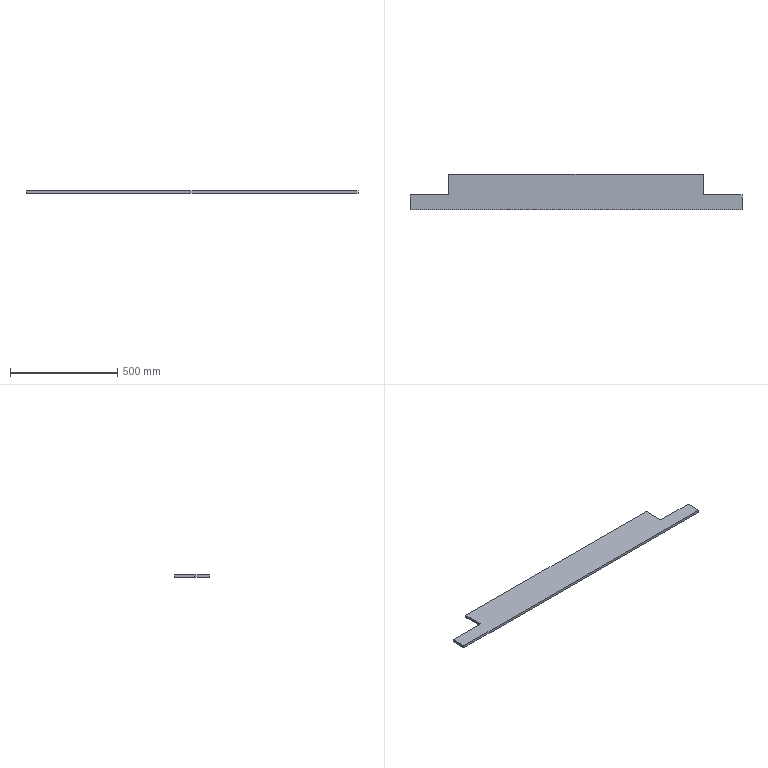Part | SolidWorks | features BaseBody 1 | 1 solid | 10 faces | box 1550 x 167 x 12 mm | volume 2687160 mm3 | plane 10
STEP:
#1=CARTESIAN_POINT('',(775.,-85.,-6.));
#2=VERTEX_POINT('',#1);
#3=CARTESIAN_POINT('',(775.,-15.,-6.));
#4=VERTEX_POINT('',#3);
#5=CARTESIAN_POINT('',(775.,85.,-6.));
#6=DIRECTION('',(0.,1.,0.));
#7=VECTOR('',#6,1000.);
#8=LINE('',#5,#7);
#9=EDGE_CURVE('',#2,#4,#8,.T.);
#10=ORIENTED_EDGE('',*,*,#9,.T.);
#11=CARTESIAN_POINT('',(775.,-15.,6.));
#12=VERTEX_POINT('',#11);
#13=CARTESIAN_POINT('',(775.,-15.,-8.));
#14=DIRECTION('',(0.,0.,1.));
#15=VECTOR('',#14,1000.);
#16=LINE('',#13,#15);
#17=EDGE_CURVE('',#4,#12,#16,.T.);
#18=ORIENTED_EDGE('',*,*,#17,.T.);
#19=CARTESIAN_POINT('',(775.,-85.,6.));
#20=VERTEX_POINT('',#19);
#21=CARTESIAN_POINT('',(775.,85.,6.));
#22=DIRECTION('',(0.,1.,0.));
#23=VECTOR('',#22,1000.);
#24=LINE('',#21,#23);
#25=EDGE_CURVE('',#20,#12,#24,.T.);
#26=ORIENTED_EDGE('',*,*,#25,.F.);
#27=CARTESIAN_POINT('',(775.,-85.,6.));
#28=DIRECTION('',(0.,0.,-1.));
#29=VECTOR('',#28,1000.);
#30=LINE('',#27,#29);
#31=EDGE_CURVE('',#20,#2,#30,.T.);
#32=ORIENTED_EDGE('',*,*,#31,.T.);
#33=EDGE_LOOP('',(#10,#18,#26,#32));
#34=FACE_OUTER_BOUND('',#33,.T.);
#35=CARTESIAN_POINT('',(775.,85.,6.));
#36=DIRECTION('',(-1.,0.,0.));
#37=DIRECTION('',(0.,0.,1.));
#38=AXIS2_PLACEMENT_3D('',#35,#36,#37);
#39=PLANE('',#38);
#40=ADVANCED_FACE('',(#34),#39,.F.);
#41=CARTESIAN_POINT('',(-775.,-15.,6.));
#42=VERTEX_POINT('',#41);
#43=CARTESIAN_POINT('',(-775.,-85.,6.));
#44=VERTEX_POINT('',#43);
#45=CARTESIAN_POINT('',(-775.,85.,6.));
#46=DIRECTION('',(0.,-1.,0.));
#47=VECTOR('',#46,1000.);
#48=LINE('',#45,#47);
#49=EDGE_CURVE('',#42,#44,#48,.T.);
#50=ORIENTED_EDGE('',*,*,#49,.F.);
#51=CARTESIAN_POINT('',(-775.,-15.,-6.));
#52=VERTEX_POINT('',#51);
#53=CARTESIAN_POINT('',(-775.,-15.,-8.));
#54=DIRECTION('',(0.,0.,1.));
#55=VECTOR('',#54,1000.);
#56=LINE('',#53,#55);
#57=EDGE_CURVE('',#52,#42,#56,.T.);
#58=ORIENTED_EDGE('',*,*,#57,.F.);
#59=CARTESIAN_POINT('',(-775.,-85.,-6.));
#60=VERTEX_POINT('',#59);
#61=CARTESIAN_POINT('',(-775.,85.,-6.));
#62=DIRECTION('',(0.,-1.,0.));
#63=VECTOR('',#62,1000.);
#64=LINE('',#61,#63);
#65=EDGE_CURVE('',#52,#60,#64,.T.);
#66=ORIENTED_EDGE('',*,*,#65,.T.);
#67=CARTESIAN_POINT('',(-775.,-85.,6.));
#68=DIRECTION('',(0.,0.,-1.));
#69=VECTOR('',#68,1000.);
#70=LINE('',#67,#69);
#71=EDGE_CURVE('',#44,#60,#70,.T.);
#72=ORIENTED_EDGE('',*,*,#71,.F.);
#73=EDGE_LOOP('',(#50,#58,#66,#72));
#74=FACE_OUTER_BOUND('',#73,.T.);
#75=CARTESIAN_POINT('',(-775.,85.,6.));
#76=DIRECTION('',(1.,0.,0.));
#77=DIRECTION('',(0.,0.,-1.));
#78=AXIS2_PLACEMENT_3D('',#75,#76,#77);
#79=PLANE('',#78);
#80=ADVANCED_FACE('',(#74),#79,.F.);
#81=CARTESIAN_POINT('',(-775.,-85.,-6.));
#82=DIRECTION('',(1.,0.,0.));
#83=VECTOR('',#82,1000.);
#84=LINE('',#81,#83);
#85=EDGE_CURVE('',#60,#2,#84,.T.);
#86=ORIENTED_EDGE('',*,*,#85,.T.);
#87=ORIENTED_EDGE('',*,*,#31,.F.);
#88=CARTESIAN_POINT('',(-775.,-85.,6.));
#89=DIRECTION('',(1.,0.,0.));
#90=VECTOR('',#89,1000.);
#91=LINE('',#88,#90);
#92=EDGE_CURVE('',#44,#20,#91,.T.);
#93=ORIENTED_EDGE('',*,*,#92,.F.);
#94=ORIENTED_EDGE('',*,*,#71,.T.);
#95=EDGE_LOOP('',(#86,#87,#93,#94));
#96=FACE_OUTER_BOUND('',#95,.T.);
#97=CARTESIAN_POINT('',(-775.,-85.,6.));
#98=DIRECTION('',(0.,1.,0.));
#99=DIRECTION('',(0.,0.,1.));
#100=AXIS2_PLACEMENT_3D('',#97,#98,#99);
#101=PLANE('',#100);
#102=ADVANCED_FACE('',(#96),#101,.F.);
#103=CARTESIAN_POINT('',(-595.,82.,6.));
#104=VERTEX_POINT('',#103);
#105=CARTESIAN_POINT('',(595.,82.,6.));
#106=VERTEX_POINT('',#105);
#107=CARTESIAN_POINT('',(-595.,82.,6.));
#108=DIRECTION('',(1.,0.,0.));
#109=VECTOR('',#108,1000.);
#110=LINE('',#107,#109);
#111=EDGE_CURVE('',#104,#106,#110,.T.);
#112=ORIENTED_EDGE('',*,*,#111,.F.);
#113=CARTESIAN_POINT('',(-595.,-15.,6.));
#114=VERTEX_POINT('',#113);
#115=CARTESIAN_POINT('',(-595.,-15.,6.));
#116=DIRECTION('',(0.,1.,0.));
#117=VECTOR('',#116,1000.);
#118=LINE('',#115,#117);
#119=EDGE_CURVE('',#114,#104,#118,.T.);
#120=ORIENTED_EDGE('',*,*,#119,.F.);
#121=CARTESIAN_POINT('',(-775.,-15.,6.));
#122=DIRECTION('',(1.,0.,0.));
#123=VECTOR('',#122,1000.);
#124=LINE('',#121,#123);
#125=EDGE_CURVE('',#42,#114,#124,.T.);
#126=ORIENTED_EDGE('',*,*,#125,.F.);
#127=ORIENTED_EDGE('',*,*,#49,.T.);
#128=ORIENTED_EDGE('',*,*,#92,.T.);
#129=ORIENTED_EDGE('',*,*,#25,.T.);
#130=CARTESIAN_POINT('',(595.,-15.,6.));
#131=VERTEX_POINT('',#130);
#132=CARTESIAN_POINT('',(775.,-15.,6.));
#133=DIRECTION('',(1.,0.,0.));
#134=VECTOR('',#133,1000.);
#135=LINE('',#132,#134);
#136=EDGE_CURVE('',#131,#12,#135,.T.);
#137=ORIENTED_EDGE('',*,*,#136,.F.);
#138=CARTESIAN_POINT('',(595.,-15.,6.));
#139=DIRECTION('',(0.,-1.,0.));
#140=VECTOR('',#139,1000.);
#141=LINE('',#138,#140);
#142=EDGE_CURVE('',#106,#131,#141,.T.);
#143=ORIENTED_EDGE('',*,*,#142,.F.);
#144=EDGE_LOOP('',(#112,#120,#126,#127,#128,#129,#137,#143));
#145=FACE_OUTER_BOUND('',#144,.T.);
#146=CARTESIAN_POINT('',(0.,0.,6.));
#147=DIRECTION('',(0.,0.,1.));
#148=DIRECTION('',(1.,0.,0.));
#149=AXIS2_PLACEMENT_3D('',#146,#147,#148);
#150=PLANE('',#149);
#151=ADVANCED_FACE('',(#145),#150,.T.);
#152=CARTESIAN_POINT('',(-595.,-15.,-6.));
#153=VERTEX_POINT('',#152);
#154=CARTESIAN_POINT('',(-595.,82.,-6.));
#155=VERTEX_POINT('',#154);
#156=CARTESIAN_POINT('',(-595.,0.,-6.));
#157=DIRECTION('',(0.,1.,0.));
#158=VECTOR('',#157,1000.);
#159=LINE('',#156,#158);
#160=EDGE_CURVE('',#153,#155,#159,.T.);
#161=ORIENTED_EDGE('',*,*,#160,.T.);
#162=CARTESIAN_POINT('',(595.,82.,-6.));
#163=VERTEX_POINT('',#162);
#164=CARTESIAN_POINT('',(0.,82.,-6.));
#165=DIRECTION('',(1.,0.,0.));
#166=VECTOR('',#165,1000.);
#167=LINE('',#164,#166);
#168=EDGE_CURVE('',#155,#163,#167,.T.);
#169=ORIENTED_EDGE('',*,*,#168,.T.);
#170=CARTESIAN_POINT('',(595.,-15.,-6.));
#171=VERTEX_POINT('',#170);
#172=CARTESIAN_POINT('',(595.,0.,-6.));
#173=DIRECTION('',(0.,-1.,0.));
#174=VECTOR('',#173,1000.);
#175=LINE('',#172,#174);
#176=EDGE_CURVE('',#163,#171,#175,.T.);
#177=ORIENTED_EDGE('',*,*,#176,.T.);
#178=CARTESIAN_POINT('',(0.,-15.,-6.));
#179=DIRECTION('',(1.,0.,0.));
#180=VECTOR('',#179,1000.);
#181=LINE('',#178,#180);
#182=EDGE_CURVE('',#171,#4,#181,.T.);
#183=ORIENTED_EDGE('',*,*,#182,.T.);
#184=ORIENTED_EDGE('',*,*,#9,.F.);
#185=ORIENTED_EDGE('',*,*,#85,.F.);
#186=ORIENTED_EDGE('',*,*,#65,.F.);
#187=CARTESIAN_POINT('',(0.,-15.,-6.));
#188=DIRECTION('',(1.,0.,0.));
#189=VECTOR('',#188,1000.);
#190=LINE('',#187,#189);
#191=EDGE_CURVE('',#52,#153,#190,.T.);
#192=ORIENTED_EDGE('',*,*,#191,.T.);
#193=EDGE_LOOP('',(#161,#169,#177,#183,#184,#185,#186,#192));
#194=FACE_OUTER_BOUND('',#193,.T.);
#195=CARTESIAN_POINT('',(0.,0.,-6.));
#196=DIRECTION('',(0.,0.,1.));
#197=DIRECTION('',(1.,0.,0.));
#198=AXIS2_PLACEMENT_3D('',#195,#196,#197);
#199=PLANE('',#198);
#200=ADVANCED_FACE('',(#194),#199,.F.);
#201=CARTESIAN_POINT('',(595.,-15.,-8.));
#202=DIRECTION('',(0.,0.,1.));
#203=VECTOR('',#202,1000.);
#204=LINE('',#201,#203);
#205=EDGE_CURVE('',#171,#131,#204,.T.);
#206=ORIENTED_EDGE('',*,*,#205,.T.);
#207=ORIENTED_EDGE('',*,*,#136,.T.);
#208=ORIENTED_EDGE('',*,*,#17,.F.);
#209=ORIENTED_EDGE('',*,*,#182,.F.);
#210=EDGE_LOOP('',(#206,#207,#208,#209));
#211=FACE_OUTER_BOUND('',#210,.T.);
#212=CARTESIAN_POINT('',(775.,-15.,-8.));
#213=DIRECTION('',(0.,-1.,0.));
#214=DIRECTION('',(0.,0.,-1.));
#215=AXIS2_PLACEMENT_3D('',#212,#213,#214);
#216=PLANE('',#215);
#217=ADVANCED_FACE('',(#211),#216,.F.);
#218=ORIENTED_EDGE('',*,*,#176,.F.);
#219=CARTESIAN_POINT('',(595.,82.,-8.));
#220=DIRECTION('',(0.,0.,1.));
#221=VECTOR('',#220,1000.);
#222=LINE('',#219,#221);
#223=EDGE_CURVE('',#163,#106,#222,.T.);
#224=ORIENTED_EDGE('',*,*,#223,.T.);
#225=ORIENTED_EDGE('',*,*,#142,.T.);
#226=ORIENTED_EDGE('',*,*,#205,.F.);
#227=EDGE_LOOP('',(#218,#224,#225,#226));
#228=FACE_OUTER_BOUND('',#227,.T.);
#229=CARTESIAN_POINT('',(595.,-15.,-8.));
#230=DIRECTION('',(-1.,0.,0.));
#231=DIRECTION('',(0.,-1.,0.));
#232=AXIS2_PLACEMENT_3D('',#229,#230,#231);
#233=PLANE('',#232);
#234=ADVANCED_FACE('',(#228),#233,.F.);
#235=ORIENTED_EDGE('',*,*,#119,.T.);
#236=CARTESIAN_POINT('',(-595.,82.,-8.));
#237=DIRECTION('',(0.,0.,-1.));
#238=VECTOR('',#237,1000.);
#239=LINE('',#236,#238);
#240=EDGE_CURVE('',#104,#155,#239,.T.);
#241=ORIENTED_EDGE('',*,*,#240,.T.);
#242=ORIENTED_EDGE('',*,*,#160,.F.);
#243=CARTESIAN_POINT('',(-595.,-15.,-8.));
#244=DIRECTION('',(0.,0.,1.));
#245=VECTOR('',#244,1000.);
#246=LINE('',#243,#245);
#247=EDGE_CURVE('',#153,#114,#246,.T.);
#248=ORIENTED_EDGE('',*,*,#247,.T.);
#249=EDGE_LOOP('',(#235,#241,#242,#248));
#250=FACE_OUTER_BOUND('',#249,.T.);
#251=CARTESIAN_POINT('',(-595.,-15.,-8.));
#252=DIRECTION('',(1.,0.,0.));
#253=DIRECTION('',(0.,1.,0.));
#254=AXIS2_PLACEMENT_3D('',#251,#252,#253);
#255=PLANE('',#254);
#256=ADVANCED_FACE('',(#250),#255,.F.);
#257=ORIENTED_EDGE('',*,*,#57,.T.);
#258=ORIENTED_EDGE('',*,*,#125,.T.);
#259=ORIENTED_EDGE('',*,*,#247,.F.);
#260=ORIENTED_EDGE('',*,*,#191,.F.);
#261=EDGE_LOOP('',(#257,#258,#259,#260));
#262=FACE_OUTER_BOUND('',#261,.T.);
#263=CARTESIAN_POINT('',(-775.,-15.,-8.));
#264=DIRECTION('',(0.,-1.,0.));
#265=DIRECTION('',(0.,0.,-1.));
#266=AXIS2_PLACEMENT_3D('',#263,#264,#265);
#267=PLANE('',#266);
#268=ADVANCED_FACE('',(#262),#267,.F.);
#269=ORIENTED_EDGE('',*,*,#240,.F.);
#270=ORIENTED_EDGE('',*,*,#111,.T.);
#271=ORIENTED_EDGE('',*,*,#223,.F.);
#272=ORIENTED_EDGE('',*,*,#168,.F.);
#273=EDGE_LOOP('',(#269,#270,#271,#272));
#274=FACE_OUTER_BOUND('',#273,.T.);
#275=CARTESIAN_POINT('',(0.,82.,-79.));
#276=DIRECTION('',(0.,-1.,0.));
#277=DIRECTION('',(0.,0.,-1.));
#278=AXIS2_PLACEMENT_3D('',#275,#276,#277);
#279=PLANE('',#278);
#280=ADVANCED_FACE('',(#274),#279,.F.);
#281=CLOSED_SHELL('',(#40,#80,#102,#151,#200,#217,#234,#256,#268,#280));
#282=MANIFOLD_SOLID_BREP('',#281);
#283=CARTESIAN_POINT('',(0.,0.,0.));
#284=DIRECTION('',(0.,0.,1.));
#285=DIRECTION('',(1.,0.,0.));
#286=AXIS2_PLACEMENT_3D('',#283,#284,#285);
#287=(LENGTH_UNIT()NAMED_UNIT(*)SI_UNIT(.MILLI.,.METRE.));
#288=UNCERTAINTY_MEASURE_WITH_UNIT(LENGTH_MEASURE(0.00001),#287,'','');
#289=(NAMED_UNIT(*)PLANE_ANGLE_UNIT()SI_UNIT($,.RADIAN.));
#290=(NAMED_UNIT(*)SI_UNIT($,.STERADIAN.)SOLID_ANGLE_UNIT());
#291=(GEOMETRIC_REPRESENTATION_CONTEXT(3)GLOBAL_UNCERTAINTY_ASSIGNED_CONTEXT((#288))GLOBAL_UNIT_ASSIGNED_CONTEXT((#287,#289,#290))REPRESENTATION_CONTEXT('',''));
#292=ADVANCED_BREP_SHAPE_REPRESENTATION('',(#282,#286),#291);